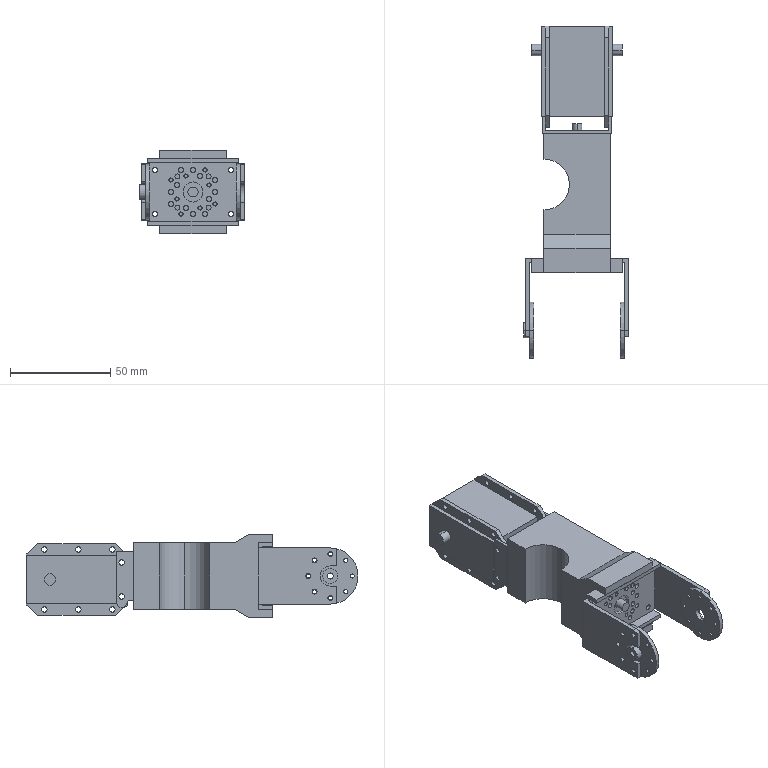Part | SolidWorks | 6 solids | 277 faces | box 52 x 166 x 41.5 mm | volume 117123 mm3 | cylinder 184 | plane 93 | commonest cylinder face diameters 2.5 x60 2.7 x40 2 x32 2.05 x16 28 x8 5 x4